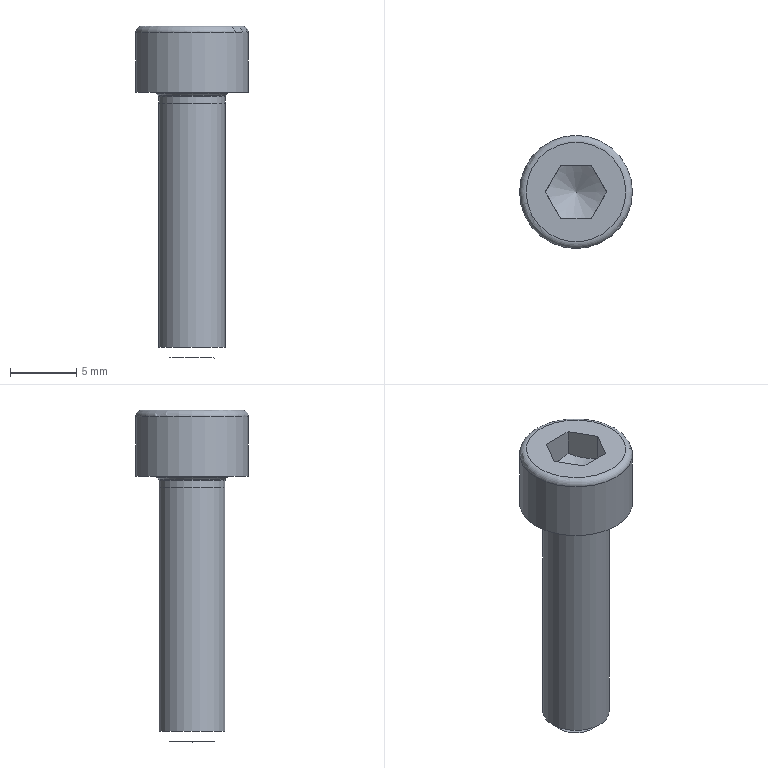Part | NX | features BREP 1, DATUM_CSYS 1 | 1 solid | 18 faces | box 8.5 x 8.5 x 25 mm | volume 636.149 mm3 | plane 9 | cone 3 | torus 3 | cylinder 3 | commonest cylinder face diameters 5 x2 8.5 x1
STEP:
#1=CARTESIAN_POINT('',(-2.309,0.,0.));
#2=VERTEX_POINT('',#1);
#3=CARTESIAN_POINT('',(-2.309,0.,-2.));
#4=VERTEX_POINT('',#3);
#5=CARTESIAN_POINT('',(-2.309,0.,0.));
#6=DIRECTION('',(0.,0.,-1.));
#7=VECTOR('',#6,1000.);
#8=LINE('',#5,#7);
#9=EDGE_CURVE('',#2,#4,#8,.T.);
#10=ORIENTED_EDGE('',*,*,#9,.T.);
#11=CARTESIAN_POINT('',(-1.155,2.,-2.));
#12=VERTEX_POINT('',#11);
#13=CARTESIAN_POINT('',(-2.309,0.,-2.));
#14=CARTESIAN_POINT('',(-1.732,1.,-2.333));
#15=CARTESIAN_POINT('',(-1.155,2.,-2.));
#16=(BOUNDED_CURVE()B_SPLINE_CURVE(2,(#13,#14,#15),.UNSPECIFIED.,.F.,.F.)B_SPLINE_CURVE_WITH_KNOTS((3,3),(0.,1.),.PIECEWISE_BEZIER_KNOTS.)CURVE()GEOMETRIC_REPRESENTATION_ITEM()RATIONAL_B_SPLINE_CURVE((1.,1.155,1.))REPRESENTATION_ITEM(''));
#17=EDGE_CURVE('',#4,#12,#16,.T.);
#18=ORIENTED_EDGE('',*,*,#17,.T.);
#19=CARTESIAN_POINT('',(-1.155,2.,0.));
#20=VERTEX_POINT('',#19);
#21=CARTESIAN_POINT('',(-1.155,2.,0.));
#22=DIRECTION('',(0.,0.,-1.));
#23=VECTOR('',#22,1000.);
#24=LINE('',#21,#23);
#25=EDGE_CURVE('',#20,#12,#24,.T.);
#26=ORIENTED_EDGE('',*,*,#25,.F.);
#27=CARTESIAN_POINT('',(-2.309,0.,0.));
#28=DIRECTION('',(0.5,0.866,0.));
#29=VECTOR('',#28,1000.);
#30=LINE('',#27,#29);
#31=EDGE_CURVE('',#2,#20,#30,.T.);
#32=ORIENTED_EDGE('',*,*,#31,.F.);
#33=EDGE_LOOP('',(#10,#18,#26,#32));
#34=FACE_BOUND('',#33,.T.);
#35=CARTESIAN_POINT('',(-1.732,1.,-1.25));
#36=DIRECTION('',(-0.866,0.5,0.));
#37=DIRECTION('',(-0.5,-0.866,0.));
#38=AXIS2_PLACEMENT_3D('',#35,#36,#37);
#39=PLANE('',#38);
#40=ADVANCED_FACE('',(#34),#39,.F.);
#41=ORIENTED_EDGE('',*,*,#25,.T.);
#42=CARTESIAN_POINT('',(1.155,2.,-2.));
#43=VERTEX_POINT('',#42);
#44=CARTESIAN_POINT('',(-1.155,2.,-2.));
#45=CARTESIAN_POINT('',(0.,2.,-2.333));
#46=CARTESIAN_POINT('',(1.155,2.,-2.));
#47=(BOUNDED_CURVE()B_SPLINE_CURVE(2,(#44,#45,#46),.UNSPECIFIED.,.F.,.F.)B_SPLINE_CURVE_WITH_KNOTS((3,3),(0.,1.),.PIECEWISE_BEZIER_KNOTS.)CURVE()GEOMETRIC_REPRESENTATION_ITEM()RATIONAL_B_SPLINE_CURVE((1.,1.155,1.))REPRESENTATION_ITEM(''));
#48=EDGE_CURVE('',#12,#43,#47,.T.);
#49=ORIENTED_EDGE('',*,*,#48,.T.);
#50=CARTESIAN_POINT('',(1.155,2.,0.));
#51=VERTEX_POINT('',#50);
#52=CARTESIAN_POINT('',(1.155,2.,0.));
#53=DIRECTION('',(0.,0.,-1.));
#54=VECTOR('',#53,1000.);
#55=LINE('',#52,#54);
#56=EDGE_CURVE('',#51,#43,#55,.T.);
#57=ORIENTED_EDGE('',*,*,#56,.F.);
#58=CARTESIAN_POINT('',(-1.155,2.,0.));
#59=DIRECTION('',(1.,0.,0.));
#60=VECTOR('',#59,1000.);
#61=LINE('',#58,#60);
#62=EDGE_CURVE('',#20,#51,#61,.T.);
#63=ORIENTED_EDGE('',*,*,#62,.F.);
#64=EDGE_LOOP('',(#41,#49,#57,#63));
#65=FACE_BOUND('',#64,.T.);
#66=CARTESIAN_POINT('',(0.,2.,-1.25));
#67=DIRECTION('',(0.,1.,0.));
#68=DIRECTION('',(-1.,0.,0.));
#69=AXIS2_PLACEMENT_3D('',#66,#67,#68);
#70=PLANE('',#69);
#71=ADVANCED_FACE('',(#65),#70,.F.);
#72=ORIENTED_EDGE('',*,*,#56,.T.);
#73=CARTESIAN_POINT('',(2.309,0.,-2.));
#74=VERTEX_POINT('',#73);
#75=CARTESIAN_POINT('',(1.155,2.,-2.));
#76=CARTESIAN_POINT('',(1.732,1.,-2.333));
#77=CARTESIAN_POINT('',(2.309,0.,-2.));
#78=(BOUNDED_CURVE()B_SPLINE_CURVE(2,(#75,#76,#77),.UNSPECIFIED.,.F.,.F.)B_SPLINE_CURVE_WITH_KNOTS((3,3),(0.,1.),.PIECEWISE_BEZIER_KNOTS.)CURVE()GEOMETRIC_REPRESENTATION_ITEM()RATIONAL_B_SPLINE_CURVE((1.,1.155,1.))REPRESENTATION_ITEM(''));
#79=EDGE_CURVE('',#43,#74,#78,.T.);
#80=ORIENTED_EDGE('',*,*,#79,.T.);
#81=CARTESIAN_POINT('',(2.309,0.,0.));
#82=VERTEX_POINT('',#81);
#83=CARTESIAN_POINT('',(2.309,0.,0.));
#84=DIRECTION('',(0.,0.,-1.));
#85=VECTOR('',#84,1000.);
#86=LINE('',#83,#85);
#87=EDGE_CURVE('',#82,#74,#86,.T.);
#88=ORIENTED_EDGE('',*,*,#87,.F.);
#89=CARTESIAN_POINT('',(1.155,2.,0.));
#90=DIRECTION('',(0.5,-0.866,0.));
#91=VECTOR('',#90,1000.);
#92=LINE('',#89,#91);
#93=EDGE_CURVE('',#51,#82,#92,.T.);
#94=ORIENTED_EDGE('',*,*,#93,.F.);
#95=EDGE_LOOP('',(#72,#80,#88,#94));
#96=FACE_BOUND('',#95,.T.);
#97=CARTESIAN_POINT('',(1.732,1.,-1.25));
#98=DIRECTION('',(0.866,0.5,0.));
#99=DIRECTION('',(-0.5,0.866,0.));
#100=AXIS2_PLACEMENT_3D('',#97,#98,#99);
#101=PLANE('',#100);
#102=ADVANCED_FACE('',(#96),#101,.F.);
#103=ORIENTED_EDGE('',*,*,#87,.T.);
#104=CARTESIAN_POINT('',(1.155,-2.,-2.));
#105=VERTEX_POINT('',#104);
#106=CARTESIAN_POINT('',(2.309,0.,-2.));
#107=CARTESIAN_POINT('',(1.732,-1.,-2.333));
#108=CARTESIAN_POINT('',(1.155,-2.,-2.));
#109=(BOUNDED_CURVE()B_SPLINE_CURVE(2,(#106,#107,#108),.UNSPECIFIED.,.F.,.F.)B_SPLINE_CURVE_WITH_KNOTS((3,3),(0.,1.),.PIECEWISE_BEZIER_KNOTS.)CURVE()GEOMETRIC_REPRESENTATION_ITEM()RATIONAL_B_SPLINE_CURVE((1.,1.155,1.))REPRESENTATION_ITEM(''));
#110=EDGE_CURVE('',#74,#105,#109,.T.);
#111=ORIENTED_EDGE('',*,*,#110,.T.);
#112=CARTESIAN_POINT('',(1.155,-2.,0.));
#113=VERTEX_POINT('',#112);
#114=CARTESIAN_POINT('',(1.155,-2.,0.));
#115=DIRECTION('',(0.,0.,-1.));
#116=VECTOR('',#115,1000.);
#117=LINE('',#114,#116);
#118=EDGE_CURVE('',#113,#105,#117,.T.);
#119=ORIENTED_EDGE('',*,*,#118,.F.);
#120=CARTESIAN_POINT('',(2.309,0.,0.));
#121=DIRECTION('',(-0.5,-0.866,0.));
#122=VECTOR('',#121,1000.);
#123=LINE('',#120,#122);
#124=EDGE_CURVE('',#82,#113,#123,.T.);
#125=ORIENTED_EDGE('',*,*,#124,.F.);
#126=EDGE_LOOP('',(#103,#111,#119,#125));
#127=FACE_BOUND('',#126,.T.);
#128=CARTESIAN_POINT('',(1.732,-1.,-1.25));
#129=DIRECTION('',(0.866,-0.5,0.));
#130=DIRECTION('',(0.5,0.866,0.));
#131=AXIS2_PLACEMENT_3D('',#128,#129,#130);
#132=PLANE('',#131);
#133=ADVANCED_FACE('',(#127),#132,.F.);
#134=ORIENTED_EDGE('',*,*,#118,.T.);
#135=CARTESIAN_POINT('',(-1.155,-2.,-2.));
#136=VERTEX_POINT('',#135);
#137=CARTESIAN_POINT('',(1.155,-2.,-2.));
#138=CARTESIAN_POINT('',(0.,-2.,-2.333));
#139=CARTESIAN_POINT('',(-1.155,-2.,-2.));
#140=(BOUNDED_CURVE()B_SPLINE_CURVE(2,(#137,#138,#139),.UNSPECIFIED.,.F.,.F.)B_SPLINE_CURVE_WITH_KNOTS((3,3),(0.,1.),.PIECEWISE_BEZIER_KNOTS.)CURVE()GEOMETRIC_REPRESENTATION_ITEM()RATIONAL_B_SPLINE_CURVE((1.,1.155,1.))REPRESENTATION_ITEM(''));
#141=EDGE_CURVE('',#105,#136,#140,.T.);
#142=ORIENTED_EDGE('',*,*,#141,.T.);
#143=CARTESIAN_POINT('',(-1.155,-2.,0.));
#144=VERTEX_POINT('',#143);
#145=CARTESIAN_POINT('',(-1.155,-2.,0.));
#146=DIRECTION('',(0.,0.,-1.));
#147=VECTOR('',#146,1000.);
#148=LINE('',#145,#147);
#149=EDGE_CURVE('',#144,#136,#148,.T.);
#150=ORIENTED_EDGE('',*,*,#149,.F.);
#151=CARTESIAN_POINT('',(1.155,-2.,0.));
#152=DIRECTION('',(-1.,0.,0.));
#153=VECTOR('',#152,1000.);
#154=LINE('',#151,#153);
#155=EDGE_CURVE('',#113,#144,#154,.T.);
#156=ORIENTED_EDGE('',*,*,#155,.F.);
#157=EDGE_LOOP('',(#134,#142,#150,#156));
#158=FACE_BOUND('',#157,.T.);
#159=CARTESIAN_POINT('',(0.,-2.,-1.25));
#160=DIRECTION('',(0.,-1.,0.));
#161=DIRECTION('',(1.,0.,0.));
#162=AXIS2_PLACEMENT_3D('',#159,#160,#161);
#163=PLANE('',#162);
#164=ADVANCED_FACE('',(#158),#163,.F.);
#165=ORIENTED_EDGE('',*,*,#149,.T.);
#166=CARTESIAN_POINT('',(-1.155,-2.,-2.));
#167=CARTESIAN_POINT('',(-1.732,-1.,-2.333));
#168=CARTESIAN_POINT('',(-2.309,0.,-2.));
#169=(BOUNDED_CURVE()B_SPLINE_CURVE(2,(#166,#167,#168),.UNSPECIFIED.,.F.,.F.)B_SPLINE_CURVE_WITH_KNOTS((3,3),(0.,1.),.PIECEWISE_BEZIER_KNOTS.)CURVE()GEOMETRIC_REPRESENTATION_ITEM()RATIONAL_B_SPLINE_CURVE((1.,1.155,1.))REPRESENTATION_ITEM(''));
#170=EDGE_CURVE('',#136,#4,#169,.T.);
#171=ORIENTED_EDGE('',*,*,#170,.T.);
#172=ORIENTED_EDGE('',*,*,#9,.F.);
#173=CARTESIAN_POINT('',(-1.155,-2.,0.));
#174=DIRECTION('',(-0.5,0.866,0.));
#175=VECTOR('',#174,1000.);
#176=LINE('',#173,#175);
#177=EDGE_CURVE('',#144,#2,#176,.T.);
#178=ORIENTED_EDGE('',*,*,#177,.F.);
#179=EDGE_LOOP('',(#165,#171,#172,#178));
#180=FACE_BOUND('',#179,.T.);
#181=CARTESIAN_POINT('',(-1.732,-1.,-1.25));
#182=DIRECTION('',(-0.866,-0.5,0.));
#183=DIRECTION('',(0.5,-0.866,0.));
#184=AXIS2_PLACEMENT_3D('',#181,#182,#183);
#185=PLANE('',#184);
#186=ADVANCED_FACE('',(#180),#185,.F.);
#187=ORIENTED_EDGE('',*,*,#79,.F.);
#188=ORIENTED_EDGE('',*,*,#48,.F.);
#189=ORIENTED_EDGE('',*,*,#17,.F.);
#190=ORIENTED_EDGE('',*,*,#170,.F.);
#191=ORIENTED_EDGE('',*,*,#141,.F.);
#192=ORIENTED_EDGE('',*,*,#110,.F.);
#193=CARTESIAN_POINT('',(0.,0.,-3.333));
#194=VERTEX_POINT('',#193);
#195=CARTESIAN_POINT('',(2.309,0.,-2.));
#196=DIRECTION('',(-0.866,0.,-0.5));
#197=VECTOR('',#196,1000.);
#198=LINE('',#195,#197);
#199=EDGE_CURVE('',#74,#194,#198,.T.);
#200=ORIENTED_EDGE('',*,*,#199,.T.);
#201=ORIENTED_EDGE('',*,*,#199,.F.);
#202=EDGE_LOOP('',(#187,#188,#189,#190,#191,#192,#200,#201));
#203=FACE_BOUND('',#202,.T.);
#204=CARTESIAN_POINT('',(0.,0.,-3.333));
#205=DIRECTION('',(0.,0.,1.));
#206=DIRECTION('',(-1.,0.,0.));
#207=AXIS2_PLACEMENT_3D('',#204,#205,#206);
#208=CONICAL_SURFACE('',#207,0.,1.047);
#209=ADVANCED_FACE('',(#203),#208,.F.);
#210=CARTESIAN_POINT('',(3.75,0.,0.));
#211=VERTEX_POINT('',#210);
#212=CARTESIAN_POINT('',(0.,0.,0.));
#213=DIRECTION('',(0.,0.,-1.));
#214=DIRECTION('',(1.,0.,0.));
#215=AXIS2_PLACEMENT_3D('',#212,#213,#214);
#216=CIRCLE('',#215,3.75);
#217=EDGE_CURVE('',#211,#211,#216,.T.);
#218=ORIENTED_EDGE('',*,*,#217,.F.);
#219=EDGE_LOOP('',(#218));
#220=FACE_BOUND('',#219,.T.);
#221=ORIENTED_EDGE('',*,*,#124,.T.);
#222=ORIENTED_EDGE('',*,*,#155,.T.);
#223=ORIENTED_EDGE('',*,*,#177,.T.);
#224=ORIENTED_EDGE('',*,*,#31,.T.);
#225=ORIENTED_EDGE('',*,*,#62,.T.);
#226=ORIENTED_EDGE('',*,*,#93,.T.);
#227=EDGE_LOOP('',(#221,#222,#223,#224,#225,#226));
#228=FACE_BOUND('',#227,.T.);
#229=CARTESIAN_POINT('',(0.,0.,0.));
#230=DIRECTION('',(0.,0.,-1.));
#231=DIRECTION('',(-1.,0.,0.));
#232=AXIS2_PLACEMENT_3D('',#229,#230,#231);
#233=PLANE('',#232);
#234=ADVANCED_FACE('',(#220,#228),#233,.F.);
#235=CARTESIAN_POINT('',(4.25,0.,-0.5));
#236=VERTEX_POINT('',#235);
#237=CARTESIAN_POINT('',(3.75,0.,-0.5));
#238=DIRECTION('',(0.,-1.,0.));
#239=DIRECTION('',(1.,0.,0.));
#240=AXIS2_PLACEMENT_3D('',#237,#238,#239);
#241=CIRCLE('',#240,0.5);
#242=EDGE_CURVE('',#236,#211,#241,.T.);
#243=ORIENTED_EDGE('',*,*,#242,.F.);
#244=CARTESIAN_POINT('',(0.,0.,-0.5));
#245=DIRECTION('',(0.,0.,-1.));
#246=DIRECTION('',(1.,0.,0.));
#247=AXIS2_PLACEMENT_3D('',#244,#245,#246);
#248=CIRCLE('',#247,4.25);
#249=EDGE_CURVE('',#236,#236,#248,.T.);
#250=ORIENTED_EDGE('',*,*,#249,.F.);
#251=ORIENTED_EDGE('',*,*,#242,.T.);
#252=ORIENTED_EDGE('',*,*,#217,.T.);
#253=EDGE_LOOP('',(#243,#250,#251,#252));
#254=FACE_BOUND('',#253,.T.);
#255=CARTESIAN_POINT('',(0.,0.,-0.5));
#256=DIRECTION('',(0.,0.,1.));
#257=DIRECTION('',(-1.,0.,0.));
#258=AXIS2_PLACEMENT_3D('',#255,#256,#257);
#259=TOROIDAL_SURFACE('',#258,3.75,0.5);
#260=ADVANCED_FACE('',(#254),#259,.T.);
#261=CARTESIAN_POINT('',(4.25,0.,-5.));
#262=VERTEX_POINT('',#261);
#263=CARTESIAN_POINT('',(0.,0.,-5.));
#264=DIRECTION('',(0.,0.,1.));
#265=DIRECTION('',(1.,0.,0.));
#266=AXIS2_PLACEMENT_3D('',#263,#264,#265);
#267=CIRCLE('',#266,4.25);
#268=EDGE_CURVE('',#262,#262,#267,.T.);
#269=ORIENTED_EDGE('',*,*,#268,.T.);
#270=CARTESIAN_POINT('',(4.25,0.,-5.));
#271=DIRECTION('',(0.,0.,1.));
#272=VECTOR('',#271,1000.);
#273=LINE('',#270,#272);
#274=EDGE_CURVE('',#262,#236,#273,.T.);
#275=ORIENTED_EDGE('',*,*,#274,.T.);
#276=ORIENTED_EDGE('',*,*,#249,.T.);
#277=ORIENTED_EDGE('',*,*,#274,.F.);
#278=EDGE_LOOP('',(#269,#275,#276,#277));
#279=FACE_BOUND('',#278,.T.);
#280=CARTESIAN_POINT('',(0.,0.,-5.));
#281=DIRECTION('',(0.,0.,1.));
#282=DIRECTION('',(-1.,0.,0.));
#283=AXIS2_PLACEMENT_3D('',#280,#281,#282);
#284=CYLINDRICAL_SURFACE('',#283,4.25);
#285=ADVANCED_FACE('',(#279),#284,.T.);
#286=ORIENTED_EDGE('',*,*,#268,.F.);
#287=EDGE_LOOP('',(#286));
#288=FACE_BOUND('',#287,.T.);
#289=CARTESIAN_POINT('',(2.84,0.,-5.));
#290=VERTEX_POINT('',#289);
#291=CARTESIAN_POINT('',(0.,0.,-5.));
#292=DIRECTION('',(0.,0.,1.));
#293=DIRECTION('',(1.,0.,0.));
#294=AXIS2_PLACEMENT_3D('',#291,#292,#293);
#295=CIRCLE('',#294,2.84);
#296=EDGE_CURVE('',#290,#290,#295,.T.);
#297=ORIENTED_EDGE('',*,*,#296,.T.);
#298=EDGE_LOOP('',(#297));
#299=FACE_BOUND('',#298,.T.);
#300=CARTESIAN_POINT('',(0.,0.,-5.));
#301=DIRECTION('',(0.,0.,1.));
#302=DIRECTION('',(-1.,0.,0.));
#303=AXIS2_PLACEMENT_3D('',#300,#301,#302);
#304=PLANE('',#303);
#305=ADVANCED_FACE('',(#288,#299),#304,.F.);
#306=CARTESIAN_POINT('',(2.699,0.,-5.059));
#307=VERTEX_POINT('',#306);
#308=CARTESIAN_POINT('',(0.,0.,-5.059));
#309=DIRECTION('',(0.,0.,1.));
#310=DIRECTION('',(1.,0.,0.));
#311=AXIS2_PLACEMENT_3D('',#308,#309,#310);
#312=CIRCLE('',#311,2.699);
#313=EDGE_CURVE('',#307,#307,#312,.T.);
#314=ORIENTED_EDGE('',*,*,#313,.T.);
#315=CARTESIAN_POINT('',(2.84,0.,-5.2));
#316=DIRECTION('',(0.,1.,0.));
#317=DIRECTION('',(-0.7071,0.,0.7071));
#318=AXIS2_PLACEMENT_3D('',#315,#316,#317);
#319=CIRCLE('',#318,0.2);
#320=EDGE_CURVE('',#307,#290,#319,.T.);
#321=ORIENTED_EDGE('',*,*,#320,.T.);
#322=ORIENTED_EDGE('',*,*,#296,.F.);
#323=ORIENTED_EDGE('',*,*,#320,.F.);
#324=EDGE_LOOP('',(#314,#321,#322,#323));
#325=FACE_BOUND('',#324,.T.);
#326=CARTESIAN_POINT('',(0.,0.,-5.2));
#327=DIRECTION('',(0.,0.,-1.));
#328=DIRECTION('',(-1.,0.,0.));
#329=AXIS2_PLACEMENT_3D('',#326,#327,#328);
#330=TOROIDAL_SURFACE('',#329,2.84,0.2);
#331=ADVANCED_FACE('',(#325),#330,.F.);
#332=CARTESIAN_POINT('',(2.559,0.,-5.199));
#333=VERTEX_POINT('',#332);
#334=CARTESIAN_POINT('',(0.,0.,-5.199));
#335=DIRECTION('',(0.,0.,1.));
#336=DIRECTION('',(1.,0.,0.));
#337=AXIS2_PLACEMENT_3D('',#334,#335,#336);
#338=CIRCLE('',#337,2.559);
#339=EDGE_CURVE('',#333,#333,#338,.T.);
#340=ORIENTED_EDGE('',*,*,#339,.T.);
#341=CARTESIAN_POINT('',(2.559,0.,-5.199));
#342=DIRECTION('',(0.7071,0.,0.7071));
#343=VECTOR('',#342,1000.);
#344=LINE('',#341,#343);
#345=EDGE_CURVE('',#333,#307,#344,.T.);
#346=ORIENTED_EDGE('',*,*,#345,.T.);
#347=ORIENTED_EDGE('',*,*,#313,.F.);
#348=ORIENTED_EDGE('',*,*,#345,.F.);
#349=EDGE_LOOP('',(#340,#346,#347,#348));
#350=FACE_BOUND('',#349,.T.);
#351=CARTESIAN_POINT('',(0.,0.,-5.199));
#352=DIRECTION('',(0.,0.,1.));
#353=DIRECTION('',(-1.,0.,0.));
#354=AXIS2_PLACEMENT_3D('',#351,#352,#353);
#355=CONICAL_SURFACE('',#354,2.559,0.7854);
#356=ADVANCED_FACE('',(#350),#355,.T.);
#357=CARTESIAN_POINT('',(2.5,0.,-5.34));
#358=VERTEX_POINT('',#357);
#359=CARTESIAN_POINT('',(0.,0.,-5.34));
#360=DIRECTION('',(0.,0.,1.));
#361=DIRECTION('',(1.,0.,0.));
#362=AXIS2_PLACEMENT_3D('',#359,#360,#361);
#363=CIRCLE('',#362,2.5);
#364=EDGE_CURVE('',#358,#358,#363,.T.);
#365=ORIENTED_EDGE('',*,*,#364,.T.);
#366=CARTESIAN_POINT('',(2.7,0.,-5.34));
#367=DIRECTION('',(0.,1.,0.));
#368=DIRECTION('',(-1.,0.,0.));
#369=AXIS2_PLACEMENT_3D('',#366,#367,#368);
#370=CIRCLE('',#369,0.2);
#371=EDGE_CURVE('',#358,#333,#370,.T.);
#372=ORIENTED_EDGE('',*,*,#371,.T.);
#373=ORIENTED_EDGE('',*,*,#339,.F.);
#374=ORIENTED_EDGE('',*,*,#371,.F.);
#375=EDGE_LOOP('',(#365,#372,#373,#374));
#376=FACE_BOUND('',#375,.T.);
#377=CARTESIAN_POINT('',(0.,0.,-5.34));
#378=DIRECTION('',(0.,0.,-1.));
#379=DIRECTION('',(-1.,0.,0.));
#380=AXIS2_PLACEMENT_3D('',#377,#378,#379);
#381=TOROIDAL_SURFACE('',#380,2.7,0.2);
#382=ADVANCED_FACE('',(#376),#381,.F.);
#383=CARTESIAN_POINT('',(2.5,0.,-5.8));
#384=VERTEX_POINT('',#383);
#385=CARTESIAN_POINT('',(0.,0.,-5.8));
#386=DIRECTION('',(0.,0.,1.));
#387=DIRECTION('',(1.,0.,0.));
#388=AXIS2_PLACEMENT_3D('',#385,#386,#387);
#389=CIRCLE('',#388,2.5);
#390=EDGE_CURVE('',#384,#384,#389,.T.);
#391=ORIENTED_EDGE('',*,*,#390,.T.);
#392=CARTESIAN_POINT('',(2.5,0.,-5.8));
#393=DIRECTION('',(0.,0.,1.));
#394=VECTOR('',#393,1000.);
#395=LINE('',#392,#394);
#396=EDGE_CURVE('',#384,#358,#395,.T.);
#397=ORIENTED_EDGE('',*,*,#396,.T.);
#398=ORIENTED_EDGE('',*,*,#364,.F.);
#399=ORIENTED_EDGE('',*,*,#396,.F.);
#400=EDGE_LOOP('',(#391,#397,#398,#399));
#401=FACE_BOUND('',#400,.T.);
#402=CARTESIAN_POINT('',(0.,0.,-5.8));
#403=DIRECTION('',(0.,0.,1.));
#404=DIRECTION('',(-1.,0.,0.));
#405=AXIS2_PLACEMENT_3D('',#402,#403,#404);
#406=CYLINDRICAL_SURFACE('',#405,2.5);
#407=ADVANCED_FACE('',(#401),#406,.T.);
#408=ORIENTED_EDGE('',*,*,#390,.F.);
#409=CARTESIAN_POINT('',(2.5,0.,-24.2));
#410=VERTEX_POINT('',#409);
#411=CARTESIAN_POINT('',(2.5,0.,-24.2));
#412=DIRECTION('',(0.,0.,1.));
#413=VECTOR('',#412,1000.);
#414=LINE('',#411,#413);
#415=EDGE_CURVE('',#410,#384,#414,.T.);
#416=ORIENTED_EDGE('',*,*,#415,.F.);
#417=CARTESIAN_POINT('',(0.,0.,-24.2));
#418=DIRECTION('',(0.,0.,-1.));
#419=DIRECTION('',(1.,0.,0.));
#420=AXIS2_PLACEMENT_3D('',#417,#418,#419);
#421=CIRCLE('',#420,2.5);
#422=EDGE_CURVE('',#410,#410,#421,.T.);
#423=ORIENTED_EDGE('',*,*,#422,.F.);
#424=ORIENTED_EDGE('',*,*,#415,.T.);
#425=EDGE_LOOP('',(#408,#416,#423,#424));
#426=FACE_BOUND('',#425,.T.);
#427=CARTESIAN_POINT('',(0.,0.,-25.));
#428=DIRECTION('',(0.,0.,1.));
#429=DIRECTION('',(-1.,0.,0.));
#430=AXIS2_PLACEMENT_3D('',#427,#428,#429);
#431=CYLINDRICAL_SURFACE('',#430,2.5);
#432=ADVANCED_FACE('',(#426),#431,.T.);
#433=CARTESIAN_POINT('',(1.7,0.,-25.));
#434=VERTEX_POINT('',#433);
#435=CARTESIAN_POINT('',(0.,0.,-25.));
#436=DIRECTION('',(0.,0.,-1.));
#437=DIRECTION('',(1.,0.,0.));
#438=AXIS2_PLACEMENT_3D('',#435,#436,#437);
#439=CIRCLE('',#438,1.7);
#440=EDGE_CURVE('',#434,#434,#439,.T.);
#441=ORIENTED_EDGE('',*,*,#440,.T.);
#442=EDGE_LOOP('',(#441));
#443=FACE_BOUND('',#442,.T.);
#444=CARTESIAN_POINT('',(0.,0.,-25.));
#445=DIRECTION('',(0.,0.,1.));
#446=DIRECTION('',(-1.,0.,0.));
#447=AXIS2_PLACEMENT_3D('',#444,#445,#446);
#448=PLANE('',#447);
#449=ADVANCED_FACE('',(#443),#448,.F.);
#450=ORIENTED_EDGE('',*,*,#440,.F.);
#451=CARTESIAN_POINT('',(1.7,0.,-25.));
#452=DIRECTION('',(0.7071,0.,0.7071));
#453=VECTOR('',#452,1000.);
#454=LINE('',#451,#453);
#455=EDGE_CURVE('',#434,#410,#454,.T.);
#456=ORIENTED_EDGE('',*,*,#455,.T.);
#457=ORIENTED_EDGE('',*,*,#422,.T.);
#458=ORIENTED_EDGE('',*,*,#455,.F.);
#459=EDGE_LOOP('',(#450,#456,#457,#458));
#460=FACE_BOUND('',#459,.T.);
#461=CARTESIAN_POINT('',(0.,0.,-25.));
#462=DIRECTION('',(0.,0.,1.));
#463=DIRECTION('',(-1.,0.,0.));
#464=AXIS2_PLACEMENT_3D('',#461,#462,#463);
#465=CONICAL_SURFACE('',#464,1.7,0.7854);
#466=ADVANCED_FACE('',(#460),#465,.T.);
#467=CLOSED_SHELL('',(#40,#71,#102,#133,#164,#186,#209,#234,#260,#285,#305,#331,#356,#382,#407,#432,#449,#466));
#468=MANIFOLD_SOLID_BREP('',#467);
#469=(LENGTH_UNIT()NAMED_UNIT(*)SI_UNIT(.MILLI.,.METRE.));
#470=UNCERTAINTY_MEASURE_WITH_UNIT(LENGTH_MEASURE(0.00001),#469,'','');
#471=(NAMED_UNIT(*)PLANE_ANGLE_UNIT()SI_UNIT($,.RADIAN.));
#472=(NAMED_UNIT(*)SI_UNIT($,.STERADIAN.)SOLID_ANGLE_UNIT());
#473=(GEOMETRIC_REPRESENTATION_CONTEXT(3)GLOBAL_UNCERTAINTY_ASSIGNED_CONTEXT((#470))GLOBAL_UNIT_ASSIGNED_CONTEXT((#469,#471,#472))REPRESENTATION_CONTEXT('',''));
#474=ADVANCED_BREP_SHAPE_REPRESENTATION('',(#468),#473);